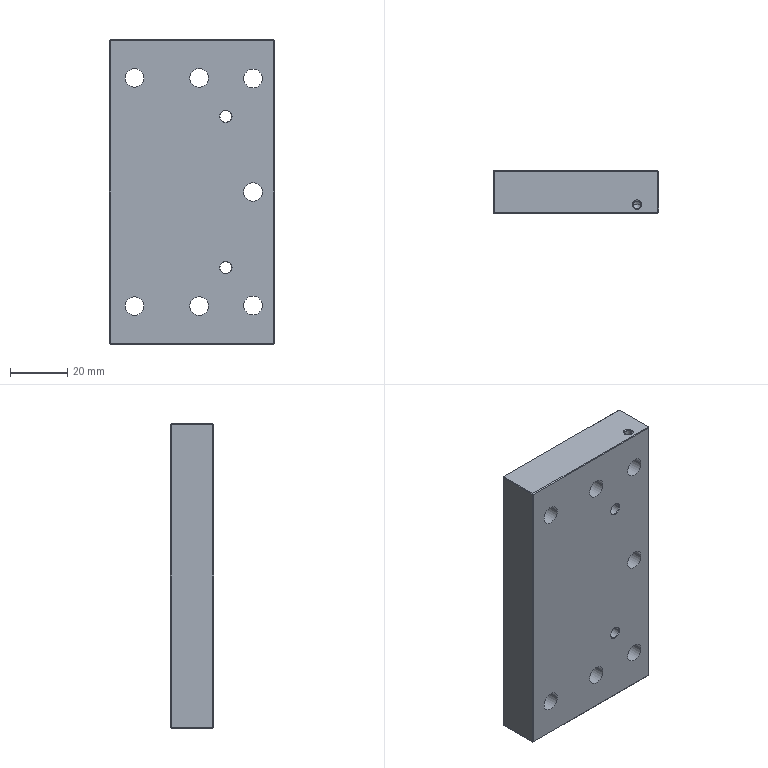Part | 1 solid | 69 faces | box 57.5 x 15 x 106 mm | volume 86278 mm3 | cylinder 28 | plane 25 | cone 16 | commonest cylinder face diameters 6.5 x14 11 x6 2.5 x4 4 x4